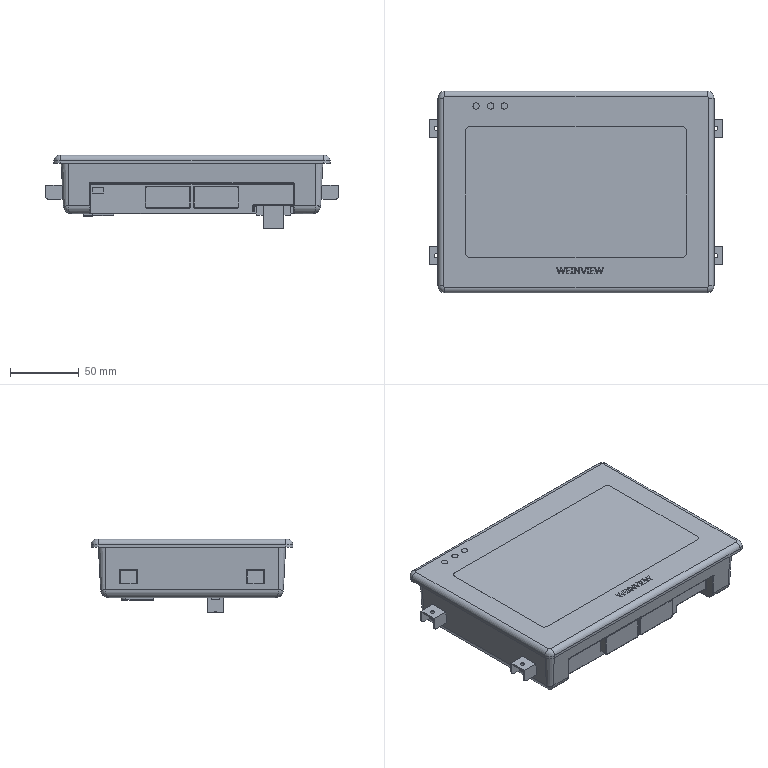Part | SolidWorks | features ICE 16, Fillet 5, MirrorPattern 2, Extrusion 1, HoleWzd 1 | 1 solid | 489 faces | box 212.35 x 146.35 x 53.56 mm | volume 1066070 mm3 | plane 282 | cylinder 101 | spline 68 | torus 22 | cone 12 | sphere 4 | commonest cylinder face diameters 1 x37 4 x14 3 x8 3.3 x8 4.541 x6 12 x5